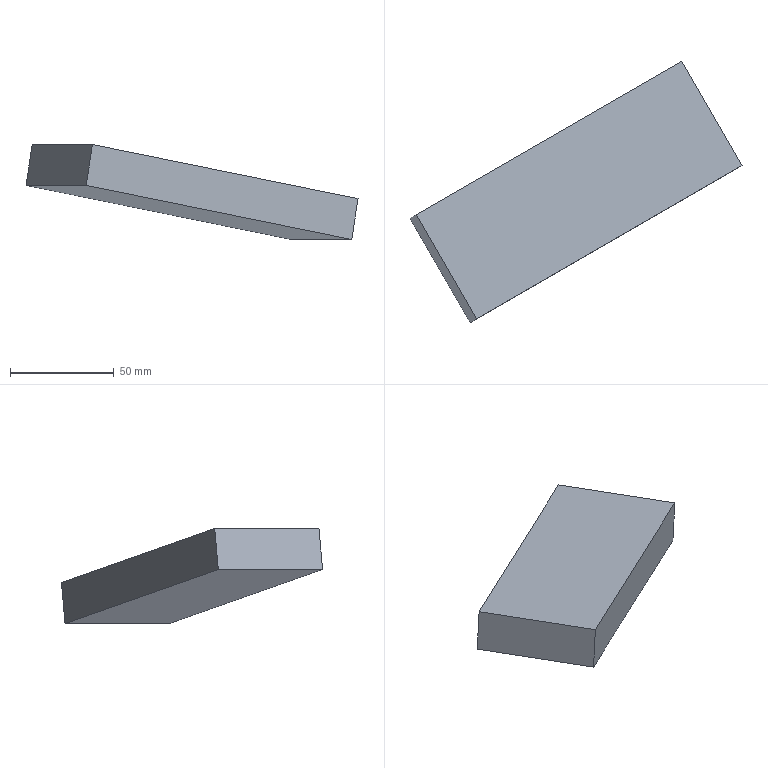Part | NX | features solid 2 | 1 solid | 6 faces | box 159.938 x 125.827 x 45.743 mm | volume 174000 mm3 | plane 6
STEP:
#1=CARTESIAN_POINT('',(-916.103,142.369,-89.317));
#2=VERTEX_POINT('',#1);
#3=CARTESIAN_POINT('',(-887.103,92.139,-89.317));
#4=VERTEX_POINT('',#3);
#5=CARTESIAN_POINT('',(-925.146,158.032,-89.317));
#6=DIRECTION('',(-0.5,0.866,0.));
#7=VECTOR('',#6,1000.);
#8=LINE('',#5,#7);
#9=EDGE_CURVE('',#2,#4,#8,.F.);
#10=ORIENTED_EDGE('',*,*,#9,.F.);
#11=CARTESIAN_POINT('',(-1044.033,68.508,-63.27));
#12=VERTEX_POINT('',#11);
#13=CARTESIAN_POINT('',(-1035.505,73.432,-65.006));
#14=DIRECTION('',(0.8529,0.4924,-0.1736));
#15=VECTOR('',#14,1000.);
#16=LINE('',#13,#15);
#17=EDGE_CURVE('',#12,#2,#16,.T.);
#18=ORIENTED_EDGE('',*,*,#17,.F.);
#19=CARTESIAN_POINT('',(-1015.033,18.279,-63.27));
#20=VERTEX_POINT('',#19);
#21=CARTESIAN_POINT('',(-1045.576,71.181,-63.27));
#22=DIRECTION('',(-0.5,0.866,0.));
#23=VECTOR('',#22,1000.);
#24=LINE('',#21,#23);
#25=EDGE_CURVE('',#12,#20,#24,.F.);
#26=ORIENTED_EDGE('',*,*,#25,.T.);
#27=CARTESIAN_POINT('',(-1006.505,23.203,-65.006));
#28=DIRECTION('',(0.8529,0.4924,-0.1736));
#29=VECTOR('',#28,1000.);
#30=LINE('',#27,#29);
#31=EDGE_CURVE('',#20,#4,#30,.T.);
#32=ORIENTED_EDGE('',*,*,#31,.T.);
#33=EDGE_LOOP('',(#10,#18,#26,#32));
#34=FACE_BOUND('',#33,.T.);
#35=CARTESIAN_POINT('',(-1037.048,76.105,-65.006));
#36=DIRECTION('',(0.1504,0.08682,0.9848));
#37=DIRECTION('',(0.8529,0.4924,-0.1736));
#38=AXIS2_PLACEMENT_3D('',#35,#36,#37);
#39=PLANE('',#38);
#40=ADVANCED_FACE('',(#34),#39,.T.);
#41=ORIENTED_EDGE('',*,*,#25,.F.);
#42=CARTESIAN_POINT('',(-1047.041,66.772,-82.966));
#43=VERTEX_POINT('',#42);
#44=CARTESIAN_POINT('',(-1047.793,66.338,-87.89));
#45=DIRECTION('',(0.1504,0.08682,0.9848));
#46=VECTOR('',#45,1000.);
#47=LINE('',#44,#46);
#48=EDGE_CURVE('',#12,#43,#47,.F.);
#49=ORIENTED_EDGE('',*,*,#48,.T.);
#50=CARTESIAN_POINT('',(-1018.041,16.542,-82.966));
#51=VERTEX_POINT('',#50);
#52=CARTESIAN_POINT('',(-1037.084,49.526,-82.966));
#53=DIRECTION('',(0.5,-0.866,0.));
#54=VECTOR('',#53,1000.);
#55=LINE('',#52,#54);
#56=EDGE_CURVE('',#43,#51,#55,.T.);
#57=ORIENTED_EDGE('',*,*,#56,.T.);
#58=CARTESIAN_POINT('',(-1018.793,16.108,-87.89));
#59=DIRECTION('',(0.1504,0.08682,0.9848));
#60=VECTOR('',#59,1000.);
#61=LINE('',#58,#60);
#62=EDGE_CURVE('',#20,#51,#61,.F.);
#63=ORIENTED_EDGE('',*,*,#62,.F.);
#64=EDGE_LOOP('',(#41,#49,#57,#63));
#65=FACE_BOUND('',#64,.T.);
#66=CARTESIAN_POINT('',(-1037.836,49.092,-87.89));
#67=DIRECTION('',(0.8529,0.4924,-0.1736));
#68=DIRECTION('',(-0.1504,-0.08682,-0.9848));
#69=AXIS2_PLACEMENT_3D('',#66,#67,#68);
#70=PLANE('',#69);
#71=ADVANCED_FACE('',(#65),#70,.F.);
#72=ORIENTED_EDGE('',*,*,#56,.F.);
#73=CARTESIAN_POINT('',(-919.111,140.632,-109.013));
#74=VERTEX_POINT('',#73);
#75=CARTESIAN_POINT('',(-1038.512,71.696,-84.702));
#76=DIRECTION('',(-0.8529,-0.4924,0.1736));
#77=VECTOR('',#76,1000.);
#78=LINE('',#75,#77);
#79=EDGE_CURVE('',#43,#74,#78,.F.);
#80=ORIENTED_EDGE('',*,*,#79,.T.);
#81=CARTESIAN_POINT('',(-890.111,90.403,-109.013));
#82=VERTEX_POINT('',#81);
#83=CARTESIAN_POINT('',(-920.654,143.305,-109.013));
#84=DIRECTION('',(0.5,-0.866,0.));
#85=VECTOR('',#84,1000.);
#86=LINE('',#83,#85);
#87=EDGE_CURVE('',#74,#82,#86,.T.);
#88=ORIENTED_EDGE('',*,*,#87,.T.);
#89=CARTESIAN_POINT('',(-1009.512,21.466,-84.702));
#90=DIRECTION('',(-0.8529,-0.4924,0.1736));
#91=VECTOR('',#90,1000.);
#92=LINE('',#89,#91);
#93=EDGE_CURVE('',#51,#82,#92,.F.);
#94=ORIENTED_EDGE('',*,*,#93,.F.);
#95=EDGE_LOOP('',(#72,#80,#88,#94));
#96=FACE_BOUND('',#95,.T.);
#97=CARTESIAN_POINT('',(-1040.055,74.368,-84.702));
#98=DIRECTION('',(0.1504,0.08682,0.9848));
#99=DIRECTION('',(0.8529,0.4924,-0.1736));
#100=AXIS2_PLACEMENT_3D('',#97,#98,#99);
#101=PLANE('',#100);
#102=ADVANCED_FACE('',(#96),#101,.F.);
#103=ORIENTED_EDGE('',*,*,#93,.T.);
#104=CARTESIAN_POINT('',(-887.103,92.139,-89.317));
#105=DIRECTION('',(0.1504,0.08682,0.9848));
#106=VECTOR('',#105,1000.);
#107=LINE('',#104,#106);
#108=EDGE_CURVE('',#4,#82,#107,.F.);
#109=ORIENTED_EDGE('',*,*,#108,.F.);
#110=ORIENTED_EDGE('',*,*,#31,.F.);
#111=ORIENTED_EDGE('',*,*,#62,.T.);
#112=EDGE_LOOP('',(#103,#109,#110,#111));
#113=FACE_BOUND('',#112,.T.);
#114=CARTESIAN_POINT('',(-1006.505,23.203,-65.006));
#115=DIRECTION('',(-0.5,0.866,0.));
#116=DIRECTION('',(-0.8627,-0.4981,0.08716));
#117=AXIS2_PLACEMENT_3D('',#114,#115,#116);
#118=PLANE('',#117);
#119=ADVANCED_FACE('',(#113),#118,.F.);
#120=CARTESIAN_POINT('',(-916.103,142.369,-89.317));
#121=DIRECTION('',(0.1504,0.08682,0.9848));
#122=VECTOR('',#121,1000.);
#123=LINE('',#120,#122);
#124=EDGE_CURVE('',#2,#74,#123,.F.);
#125=ORIENTED_EDGE('',*,*,#124,.F.);
#126=ORIENTED_EDGE('',*,*,#9,.T.);
#127=ORIENTED_EDGE('',*,*,#108,.T.);
#128=ORIENTED_EDGE('',*,*,#87,.F.);
#129=EDGE_LOOP('',(#125,#126,#127,#128));
#130=FACE_BOUND('',#129,.T.);
#131=CARTESIAN_POINT('',(-928.906,155.861,-113.937));
#132=DIRECTION('',(-0.8529,-0.4924,0.1736));
#133=DIRECTION('',(0.1504,0.08682,0.9848));
#134=AXIS2_PLACEMENT_3D('',#131,#132,#133);
#135=PLANE('',#134);
#136=ADVANCED_FACE('',(#130),#135,.F.);
#137=ORIENTED_EDGE('',*,*,#79,.F.);
#138=ORIENTED_EDGE('',*,*,#48,.F.);
#139=ORIENTED_EDGE('',*,*,#17,.T.);
#140=ORIENTED_EDGE('',*,*,#124,.T.);
#141=EDGE_LOOP('',(#137,#138,#139,#140));
#142=FACE_BOUND('',#141,.T.);
#143=CARTESIAN_POINT('',(-1035.505,73.432,-65.006));
#144=DIRECTION('',(-0.5,0.866,0.));
#145=DIRECTION('',(-0.8627,-0.4981,0.08716));
#146=AXIS2_PLACEMENT_3D('',#143,#144,#145);
#147=PLANE('',#146);
#148=ADVANCED_FACE('',(#142),#147,.T.);
#149=CLOSED_SHELL('',(#40,#71,#102,#119,#136,#148));
#150=MANIFOLD_SOLID_BREP('',#149);
#151=(LENGTH_UNIT()NAMED_UNIT(*)SI_UNIT(.MILLI.,.METRE.));
#152=UNCERTAINTY_MEASURE_WITH_UNIT(LENGTH_MEASURE(0.00001),#151,'','');
#153=(NAMED_UNIT(*)PLANE_ANGLE_UNIT()SI_UNIT($,.RADIAN.));
#154=(NAMED_UNIT(*)SI_UNIT($,.STERADIAN.)SOLID_ANGLE_UNIT());
#155=(GEOMETRIC_REPRESENTATION_CONTEXT(3)GLOBAL_UNCERTAINTY_ASSIGNED_CONTEXT((#152))GLOBAL_UNIT_ASSIGNED_CONTEXT((#151,#153,#154))REPRESENTATION_CONTEXT('',''));
#156=ADVANCED_BREP_SHAPE_REPRESENTATION('',(#150),#155);